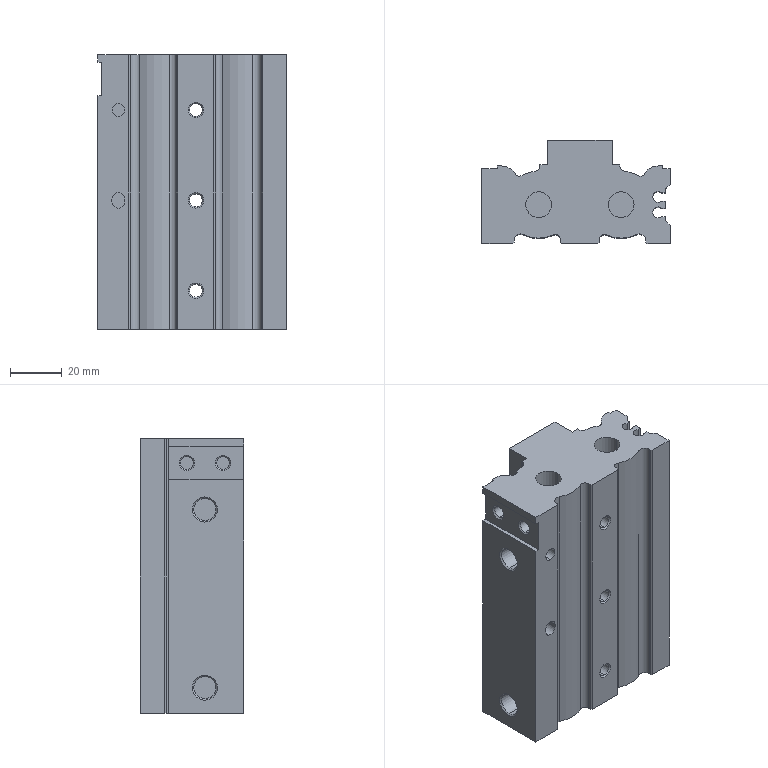Part | STEP file | _MXS20-50(0)_BODY_1 | 1 solid | 165 faces | box 73 x 40 x 106.5 mm | volume 190258 mm3 | cylinder 71 | plane 68 | cone 26 | commonest cylinder face diameters 4.134 x12 4.917 x10 5 x7 4 x6 5.1 x6 9.5 x6